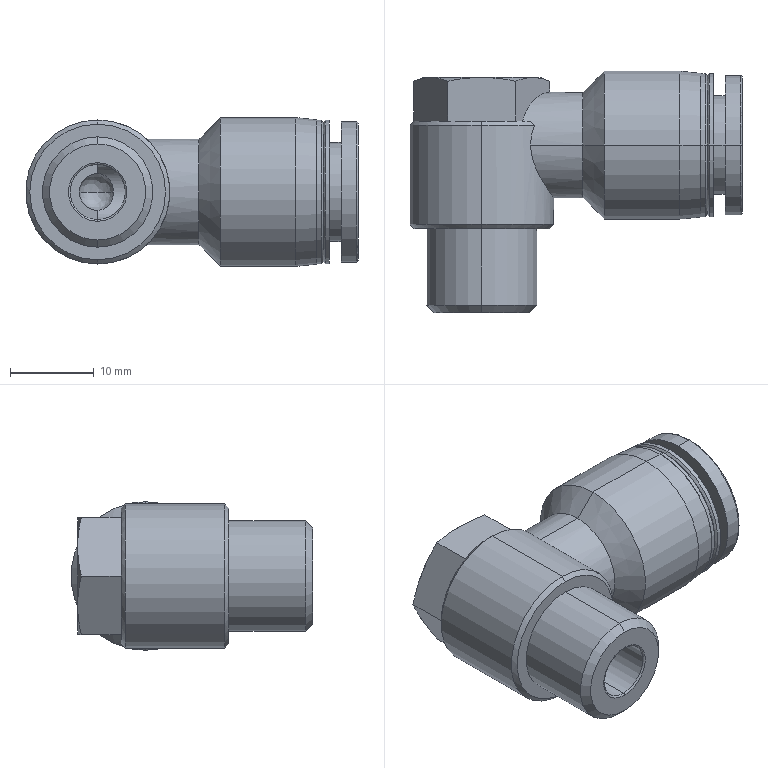Part | STEP file | 1 solid | 75 faces | box 39.583 x 28.8 x 17.7 mm | volume 7284 mm3 | cylinder 23 | plane 23 | cone 21 | torus 6 | spline 2 | commonest cylinder face diameters 17.1 x4 6.579 x2 6.667 x2 10 x2 11.8 x2 12.6 x2